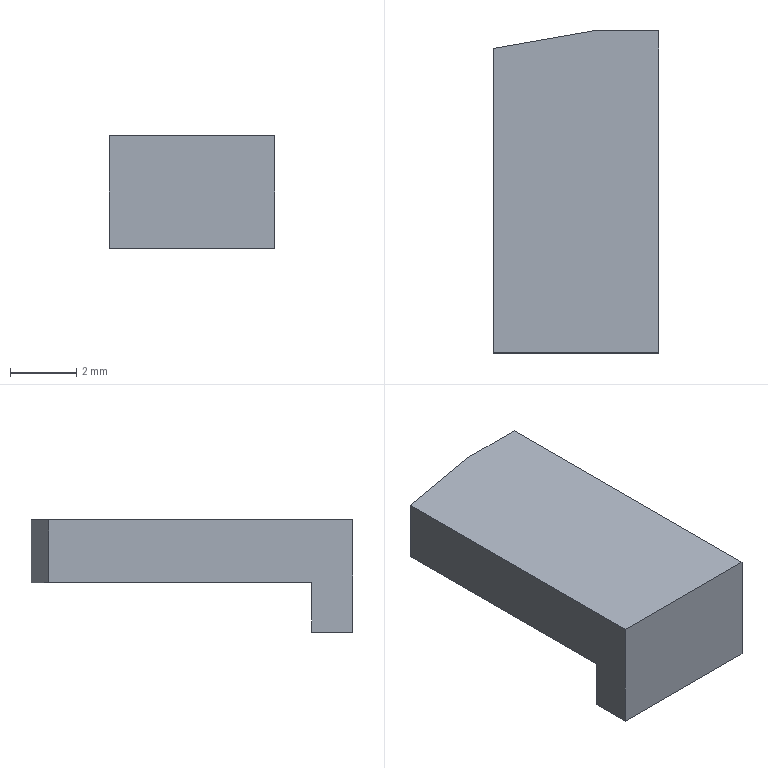Part | NX | 1 solid | 9 faces | box 5 x 9.75 x 3.4 mm | volume 100.492 mm3 | plane 9
STEP:
#1=CARTESIAN_POINT('',(-20.11,-56.129,7.853));
#2=VERTEX_POINT('',#1);
#3=CARTESIAN_POINT('',(-20.11,-64.629,7.853));
#4=VERTEX_POINT('',#3);
#5=CARTESIAN_POINT('',(-20.11,-63.129,7.853));
#6=DIRECTION('',(0.,-1.,0.));
#7=VECTOR('',#6,1000.);
#8=LINE('',#5,#7);
#9=EDGE_CURVE('',#2,#4,#8,.T.);
#10=ORIENTED_EDGE('',*,*,#9,.T.);
#11=CARTESIAN_POINT('',(-25.11,-64.629,7.853));
#12=VERTEX_POINT('',#11);
#13=CARTESIAN_POINT('',(-22.513,-64.629,7.853));
#14=DIRECTION('',(1.,0.,0.));
#15=VECTOR('',#14,1000.);
#16=LINE('',#13,#15);
#17=EDGE_CURVE('',#12,#4,#16,.T.);
#18=ORIENTED_EDGE('',*,*,#17,.F.);
#19=CARTESIAN_POINT('',(-25.11,-56.658,7.853));
#20=VERTEX_POINT('',#19);
#21=CARTESIAN_POINT('',(-25.11,-63.129,7.853));
#22=DIRECTION('',(0.,1.,0.));
#23=VECTOR('',#22,1000.);
#24=LINE('',#21,#23);
#25=EDGE_CURVE('',#12,#20,#24,.T.);
#26=ORIENTED_EDGE('',*,*,#25,.T.);
#27=CARTESIAN_POINT('',(-22.11,-56.129,7.853));
#28=VERTEX_POINT('',#27);
#29=CARTESIAN_POINT('',(-22.513,-56.2,7.853));
#30=DIRECTION('',(0.9848,0.1736,0.));
#31=VECTOR('',#30,1000.);
#32=LINE('',#29,#31);
#33=EDGE_CURVE('',#20,#28,#32,.T.);
#34=ORIENTED_EDGE('',*,*,#33,.T.);
#35=CARTESIAN_POINT('',(-22.513,-56.129,7.853));
#36=DIRECTION('',(1.,0.,0.));
#37=VECTOR('',#36,1000.);
#38=LINE('',#35,#37);
#39=EDGE_CURVE('',#28,#2,#38,.T.);
#40=ORIENTED_EDGE('',*,*,#39,.T.);
#41=EDGE_LOOP('',(#10,#18,#26,#34,#40));
#42=FACE_BOUND('',#41,.T.);
#43=CARTESIAN_POINT('',(-32.11,-63.129,7.853));
#44=DIRECTION('',(0.,0.,-1.));
#45=DIRECTION('',(0.,-1.,0.));
#46=AXIS2_PLACEMENT_3D('',#43,#44,#45);
#47=PLANE('',#46);
#48=ADVANCED_FACE('',(#42),#47,.T.);
#49=CARTESIAN_POINT('',(-25.11,-65.879,6.353));
#50=VERTEX_POINT('',#49);
#51=CARTESIAN_POINT('',(-25.11,-65.879,9.753));
#52=VERTEX_POINT('',#51);
#53=CARTESIAN_POINT('',(-25.11,-65.879,13.966));
#54=DIRECTION('',(0.,0.,1.));
#55=VECTOR('',#54,1000.);
#56=LINE('',#53,#55);
#57=EDGE_CURVE('',#50,#52,#56,.T.);
#58=ORIENTED_EDGE('',*,*,#57,.T.);
#59=CARTESIAN_POINT('',(-25.11,-56.658,9.753));
#60=VERTEX_POINT('',#59);
#61=CARTESIAN_POINT('',(-25.11,-63.129,9.753));
#62=DIRECTION('',(0.,-1.,0.));
#63=VECTOR('',#62,1000.);
#64=LINE('',#61,#63);
#65=EDGE_CURVE('',#60,#52,#64,.T.);
#66=ORIENTED_EDGE('',*,*,#65,.F.);
#67=CARTESIAN_POINT('',(-25.11,-56.658,8.803));
#68=DIRECTION('',(0.,0.,-1.));
#69=VECTOR('',#68,1000.);
#70=LINE('',#67,#69);
#71=EDGE_CURVE('',#60,#20,#70,.T.);
#72=ORIENTED_EDGE('',*,*,#71,.T.);
#73=ORIENTED_EDGE('',*,*,#25,.F.);
#74=CARTESIAN_POINT('',(-25.11,-64.629,6.353));
#75=VERTEX_POINT('',#74);
#76=CARTESIAN_POINT('',(-25.11,-64.629,13.966));
#77=DIRECTION('',(0.,0.,-1.));
#78=VECTOR('',#77,1000.);
#79=LINE('',#76,#78);
#80=EDGE_CURVE('',#12,#75,#79,.T.);
#81=ORIENTED_EDGE('',*,*,#80,.T.);
#82=CARTESIAN_POINT('',(-25.11,-63.129,6.353));
#83=DIRECTION('',(0.,1.,0.));
#84=VECTOR('',#83,1000.);
#85=LINE('',#82,#84);
#86=EDGE_CURVE('',#50,#75,#85,.T.);
#87=ORIENTED_EDGE('',*,*,#86,.F.);
#88=EDGE_LOOP('',(#58,#66,#72,#73,#81,#87));
#89=FACE_BOUND('',#88,.T.);
#90=CARTESIAN_POINT('',(-25.11,-63.129,9.253));
#91=DIRECTION('',(-1.,0.,0.));
#92=DIRECTION('',(0.,0.,1.));
#93=AXIS2_PLACEMENT_3D('',#90,#91,#92);
#94=PLANE('',#93);
#95=ADVANCED_FACE('',(#89),#94,.T.);
#96=CARTESIAN_POINT('',(-20.11,-56.129,9.753));
#97=VERTEX_POINT('',#96);
#98=CARTESIAN_POINT('',(-22.11,-56.129,9.753));
#99=VERTEX_POINT('',#98);
#100=CARTESIAN_POINT('',(-22.513,-56.129,9.753));
#101=DIRECTION('',(-1.,0.,0.));
#102=VECTOR('',#101,1000.);
#103=LINE('',#100,#102);
#104=EDGE_CURVE('',#97,#99,#103,.T.);
#105=ORIENTED_EDGE('',*,*,#104,.T.);
#106=CARTESIAN_POINT('',(-22.513,-56.2,9.753));
#107=DIRECTION('',(-0.9848,-0.1736,0.));
#108=VECTOR('',#107,1000.);
#109=LINE('',#106,#108);
#110=EDGE_CURVE('',#99,#60,#109,.T.);
#111=ORIENTED_EDGE('',*,*,#110,.T.);
#112=ORIENTED_EDGE('',*,*,#65,.T.);
#113=CARTESIAN_POINT('',(-20.11,-65.879,9.753));
#114=VERTEX_POINT('',#113);
#115=CARTESIAN_POINT('',(-22.513,-65.879,9.753));
#116=DIRECTION('',(1.,0.,0.));
#117=VECTOR('',#116,1000.);
#118=LINE('',#115,#117);
#119=EDGE_CURVE('',#52,#114,#118,.T.);
#120=ORIENTED_EDGE('',*,*,#119,.T.);
#121=CARTESIAN_POINT('',(-20.11,-63.129,9.753));
#122=DIRECTION('',(0.,1.,0.));
#123=VECTOR('',#122,1000.);
#124=LINE('',#121,#123);
#125=EDGE_CURVE('',#114,#97,#124,.T.);
#126=ORIENTED_EDGE('',*,*,#125,.T.);
#127=EDGE_LOOP('',(#105,#111,#112,#120,#126));
#128=FACE_BOUND('',#127,.T.);
#129=CARTESIAN_POINT('',(-16.11,-63.129,9.753));
#130=DIRECTION('',(0.,0.,1.));
#131=DIRECTION('',(1.,0.,0.));
#132=AXIS2_PLACEMENT_3D('',#129,#130,#131);
#133=PLANE('',#132);
#134=ADVANCED_FACE('',(#128),#133,.T.);
#135=CARTESIAN_POINT('',(-20.11,-56.129,13.966));
#136=DIRECTION('',(0.,0.,1.));
#137=VECTOR('',#136,1000.);
#138=LINE('',#135,#137);
#139=EDGE_CURVE('',#2,#97,#138,.T.);
#140=ORIENTED_EDGE('',*,*,#139,.T.);
#141=ORIENTED_EDGE('',*,*,#125,.F.);
#142=CARTESIAN_POINT('',(-20.11,-65.879,6.353));
#143=VERTEX_POINT('',#142);
#144=CARTESIAN_POINT('',(-20.11,-65.879,13.966));
#145=DIRECTION('',(0.,0.,1.));
#146=VECTOR('',#145,1000.);
#147=LINE('',#144,#146);
#148=EDGE_CURVE('',#143,#114,#147,.T.);
#149=ORIENTED_EDGE('',*,*,#148,.F.);
#150=CARTESIAN_POINT('',(-20.11,-64.629,6.353));
#151=VERTEX_POINT('',#150);
#152=CARTESIAN_POINT('',(-20.11,-63.129,6.353));
#153=DIRECTION('',(0.,-1.,0.));
#154=VECTOR('',#153,1000.);
#155=LINE('',#152,#154);
#156=EDGE_CURVE('',#151,#143,#155,.T.);
#157=ORIENTED_EDGE('',*,*,#156,.F.);
#158=CARTESIAN_POINT('',(-20.11,-64.629,13.966));
#159=DIRECTION('',(0.,0.,-1.));
#160=VECTOR('',#159,1000.);
#161=LINE('',#158,#160);
#162=EDGE_CURVE('',#4,#151,#161,.T.);
#163=ORIENTED_EDGE('',*,*,#162,.F.);
#164=ORIENTED_EDGE('',*,*,#9,.F.);
#165=EDGE_LOOP('',(#140,#141,#149,#157,#163,#164));
#166=FACE_BOUND('',#165,.T.);
#167=CARTESIAN_POINT('',(-20.11,-63.129,7.853));
#168=DIRECTION('',(1.,0.,0.));
#169=DIRECTION('',(0.,-1.,0.));
#170=AXIS2_PLACEMENT_3D('',#167,#168,#169);
#171=PLANE('',#170);
#172=ADVANCED_FACE('',(#166),#171,.T.);
#173=ORIENTED_EDGE('',*,*,#156,.T.);
#174=CARTESIAN_POINT('',(-22.513,-65.879,6.353));
#175=DIRECTION('',(-1.,0.,0.));
#176=VECTOR('',#175,1000.);
#177=LINE('',#174,#176);
#178=EDGE_CURVE('',#143,#50,#177,.T.);
#179=ORIENTED_EDGE('',*,*,#178,.T.);
#180=ORIENTED_EDGE('',*,*,#86,.T.);
#181=CARTESIAN_POINT('',(-22.513,-64.629,6.353));
#182=DIRECTION('',(1.,0.,0.));
#183=VECTOR('',#182,1000.);
#184=LINE('',#181,#183);
#185=EDGE_CURVE('',#75,#151,#184,.T.);
#186=ORIENTED_EDGE('',*,*,#185,.T.);
#187=EDGE_LOOP('',(#173,#179,#180,#186));
#188=FACE_BOUND('',#187,.T.);
#189=CARTESIAN_POINT('',(-19.282,-63.809,6.353));
#190=DIRECTION('',(0.,0.,-1.));
#191=DIRECTION('',(0.,-1.,0.));
#192=AXIS2_PLACEMENT_3D('',#189,#190,#191);
#193=PLANE('',#192);
#194=ADVANCED_FACE('',(#188),#193,.T.);
#195=CARTESIAN_POINT('',(-22.11,-56.129,8.803));
#196=DIRECTION('',(0.,0.,-1.));
#197=VECTOR('',#196,1000.);
#198=LINE('',#195,#197);
#199=EDGE_CURVE('',#99,#28,#198,.T.);
#200=ORIENTED_EDGE('',*,*,#199,.F.);
#201=ORIENTED_EDGE('',*,*,#104,.F.);
#202=ORIENTED_EDGE('',*,*,#139,.F.);
#203=ORIENTED_EDGE('',*,*,#39,.F.);
#204=EDGE_LOOP('',(#200,#201,#202,#203));
#205=FACE_BOUND('',#204,.T.);
#206=CARTESIAN_POINT('',(-22.513,-56.129,13.966));
#207=DIRECTION('',(0.,-1.,0.));
#208=DIRECTION('',(-1.,0.,0.));
#209=AXIS2_PLACEMENT_3D('',#206,#207,#208);
#210=PLANE('',#209);
#211=ADVANCED_FACE('',(#205),#210,.F.);
#212=ORIENTED_EDGE('',*,*,#199,.T.);
#213=ORIENTED_EDGE('',*,*,#33,.F.);
#214=ORIENTED_EDGE('',*,*,#71,.F.);
#215=ORIENTED_EDGE('',*,*,#110,.F.);
#216=EDGE_LOOP('',(#212,#213,#214,#215));
#217=FACE_BOUND('',#216,.T.);
#218=CARTESIAN_POINT('',(-23.61,-56.393,8.803));
#219=DIRECTION('',(0.1736,-0.9848,0.));
#220=DIRECTION('',(0.,0.,-1.));
#221=AXIS2_PLACEMENT_3D('',#218,#219,#220);
#222=PLANE('',#221);
#223=ADVANCED_FACE('',(#217),#222,.F.);
#224=ORIENTED_EDGE('',*,*,#57,.F.);
#225=ORIENTED_EDGE('',*,*,#178,.F.);
#226=ORIENTED_EDGE('',*,*,#148,.T.);
#227=ORIENTED_EDGE('',*,*,#119,.F.);
#228=EDGE_LOOP('',(#224,#225,#226,#227));
#229=FACE_BOUND('',#228,.T.);
#230=CARTESIAN_POINT('',(-20.513,-65.879,13.966));
#231=DIRECTION('',(0.,-1.,0.));
#232=DIRECTION('',(-1.,0.,0.));
#233=AXIS2_PLACEMENT_3D('',#230,#231,#232);
#234=PLANE('',#233);
#235=ADVANCED_FACE('',(#229),#234,.T.);
#236=ORIENTED_EDGE('',*,*,#17,.T.);
#237=ORIENTED_EDGE('',*,*,#162,.T.);
#238=ORIENTED_EDGE('',*,*,#185,.F.);
#239=ORIENTED_EDGE('',*,*,#80,.F.);
#240=EDGE_LOOP('',(#236,#237,#238,#239));
#241=FACE_BOUND('',#240,.T.);
#242=CARTESIAN_POINT('',(-16.21,-64.629,7.853));
#243=DIRECTION('',(0.,1.,0.));
#244=DIRECTION('',(1.,0.,0.));
#245=AXIS2_PLACEMENT_3D('',#242,#243,#244);
#246=PLANE('',#245);
#247=ADVANCED_FACE('',(#241),#246,.T.);
#248=CLOSED_SHELL('',(#48,#95,#134,#172,#194,#211,#223,#235,#247));
#249=MANIFOLD_SOLID_BREP('',#248);
#250=(LENGTH_UNIT()NAMED_UNIT(*)SI_UNIT(.MILLI.,.METRE.));
#251=UNCERTAINTY_MEASURE_WITH_UNIT(LENGTH_MEASURE(0.00001),#250,'','');
#252=(NAMED_UNIT(*)PLANE_ANGLE_UNIT()SI_UNIT($,.RADIAN.));
#253=(NAMED_UNIT(*)SI_UNIT($,.STERADIAN.)SOLID_ANGLE_UNIT());
#254=(GEOMETRIC_REPRESENTATION_CONTEXT(3)GLOBAL_UNCERTAINTY_ASSIGNED_CONTEXT((#251))GLOBAL_UNIT_ASSIGNED_CONTEXT((#250,#252,#253))REPRESENTATION_CONTEXT('',''));
#255=ADVANCED_BREP_SHAPE_REPRESENTATION('',(#249),#254);